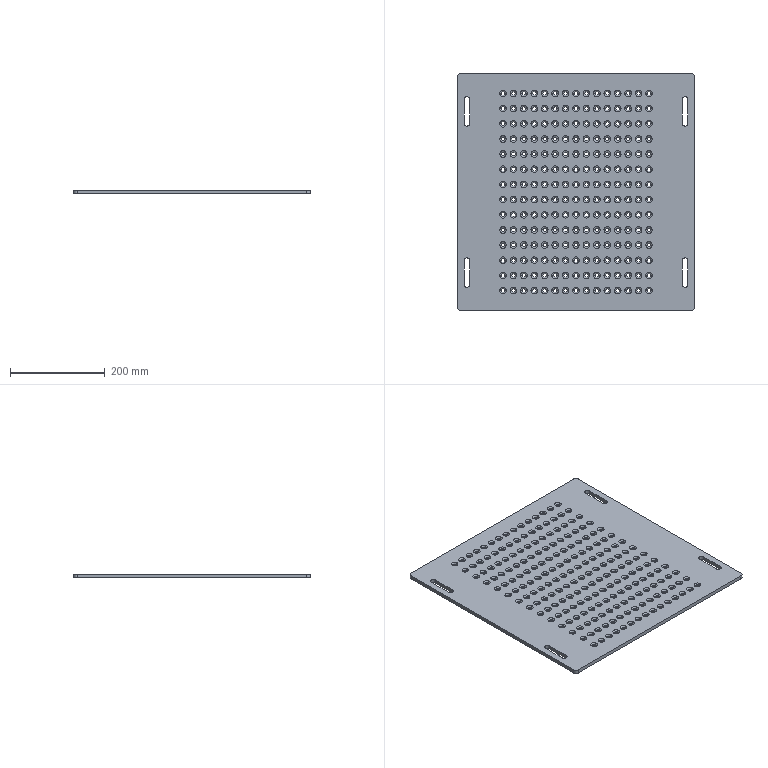Part | SolidWorks | features ICE 2, MirrorPattern 2, Extrusion 1, Fillet 1, LPattern 1 | 1 solid | 1286 faces | box 500 x 500 x 8 mm | volume 1868492 mm3 | torus 840 | cylinder 432 | plane 14 | commonest cylinder face diameters 8 x420 12 x8 16 x4